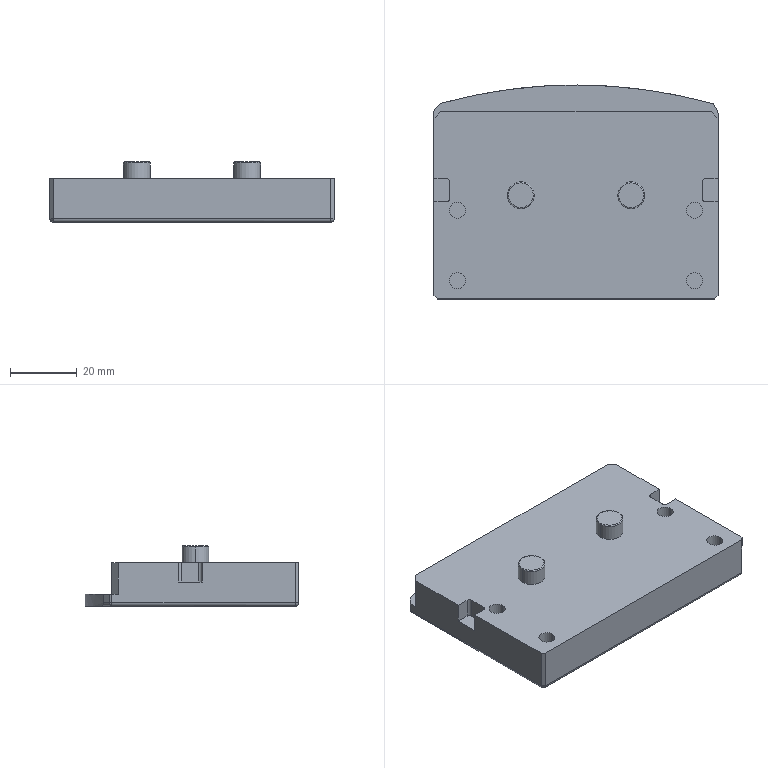Part | SolidWorks | features BaseBody 1 | 1 solid | 104 faces | box 85 x 64 x 18 mm | volume 62222 mm3 | cylinder 52 | plane 42 | spline 6 | cone 4 | commonest cylinder face diameters 2 x17 8 x12 4.8 x8 7 x8 3.3 x4 14 x2